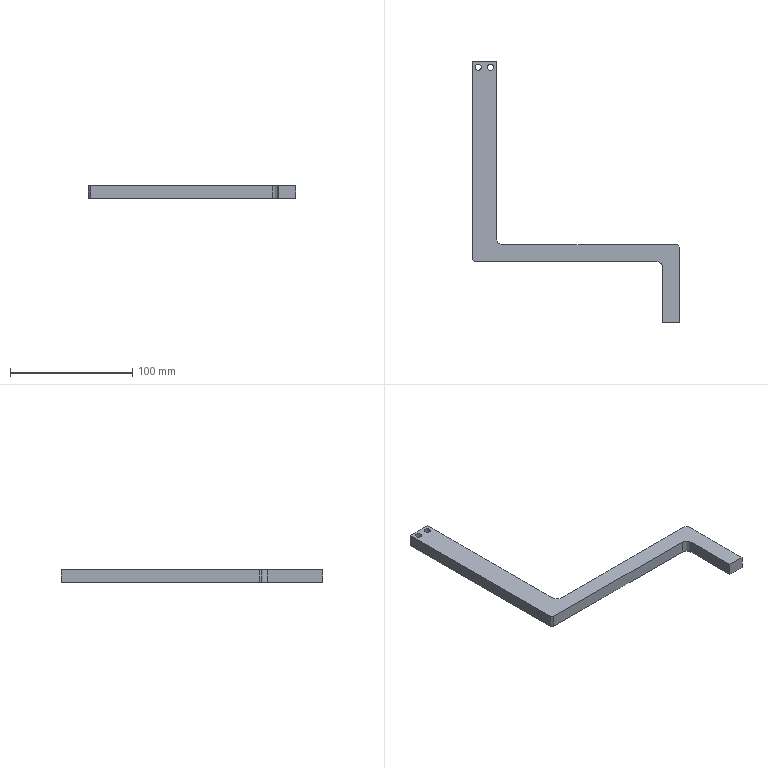Part | SolidWorks | features ICE 2, Chamfer 1, Extrusion 1, Fillet 1 | 1 solid | 18 faces | box 170 x 214 x 10 mm | volume 60475 mm3 | plane 12 | cylinder 6 | commonest cylinder face diameters 5 x4 10 x2
STEP:
#1=CARTESIAN_POINT('',(-82.5,159.,-5.));
#2=VERTEX_POINT('',#1);
#3=CARTESIAN_POINT('',(-77.5,159.,-5.));
#4=VERTEX_POINT('',#3);
#5=CARTESIAN_POINT('',(-80.,159.,-5.));
#6=DIRECTION('',(0.,0.,1.));
#7=DIRECTION('',(-1.,0.,0.));
#8=AXIS2_PLACEMENT_3D('',#5,#6,#7);
#9=CIRCLE('',#8,2.5);
#10=EDGE_CURVE('',#2,#4,#9,.T.);
#11=ORIENTED_EDGE('',*,*,#10,.F.);
#12=CARTESIAN_POINT('',(-82.5,159.,5.));
#13=VERTEX_POINT('',#12);
#14=CARTESIAN_POINT('',(-82.5,159.,-5.001));
#15=DIRECTION('',(0.,0.,1.));
#16=VECTOR('',#15,1000.);
#17=LINE('',#14,#16);
#18=EDGE_CURVE('',#2,#13,#17,.T.);
#19=ORIENTED_EDGE('',*,*,#18,.T.);
#20=CARTESIAN_POINT('',(-77.5,159.,5.));
#21=VERTEX_POINT('',#20);
#22=CARTESIAN_POINT('',(-80.,159.,5.));
#23=DIRECTION('',(0.,0.,1.));
#24=DIRECTION('',(1.,0.,0.));
#25=AXIS2_PLACEMENT_3D('',#22,#23,#24);
#26=CIRCLE('',#25,2.5);
#27=EDGE_CURVE('',#13,#21,#26,.T.);
#28=ORIENTED_EDGE('',*,*,#27,.T.);
#29=CARTESIAN_POINT('',(-77.5,159.,-5.001));
#30=DIRECTION('',(0.,0.,1.));
#31=VECTOR('',#30,1000.);
#32=LINE('',#29,#31);
#33=EDGE_CURVE('',#4,#21,#32,.T.);
#34=ORIENTED_EDGE('',*,*,#33,.F.);
#35=EDGE_LOOP('',(#11,#19,#28,#34));
#36=FACE_OUTER_BOUND('',#35,.T.);
#37=CARTESIAN_POINT('',(-80.,159.,-5.001));
#38=DIRECTION('',(0.,0.,1.));
#39=DIRECTION('',(1.,0.,0.));
#40=AXIS2_PLACEMENT_3D('',#37,#38,#39);
#41=CYLINDRICAL_SURFACE('',#40,2.5);
#42=ADVANCED_FACE('',(#36),#41,.F.);
#43=CARTESIAN_POINT('',(-72.5,159.,-5.));
#44=VERTEX_POINT('',#43);
#45=CARTESIAN_POINT('',(-67.5,159.,-5.));
#46=VERTEX_POINT('',#45);
#47=CARTESIAN_POINT('',(-70.,159.,-5.));
#48=DIRECTION('',(0.,0.,1.));
#49=DIRECTION('',(-1.,0.,0.));
#50=AXIS2_PLACEMENT_3D('',#47,#48,#49);
#51=CIRCLE('',#50,2.5);
#52=EDGE_CURVE('',#44,#46,#51,.T.);
#53=ORIENTED_EDGE('',*,*,#52,.F.);
#54=CARTESIAN_POINT('',(-72.5,159.,5.));
#55=VERTEX_POINT('',#54);
#56=CARTESIAN_POINT('',(-72.5,159.,-5.001));
#57=DIRECTION('',(0.,0.,1.));
#58=VECTOR('',#57,1000.);
#59=LINE('',#56,#58);
#60=EDGE_CURVE('',#44,#55,#59,.T.);
#61=ORIENTED_EDGE('',*,*,#60,.T.);
#62=CARTESIAN_POINT('',(-67.5,159.,5.));
#63=VERTEX_POINT('',#62);
#64=CARTESIAN_POINT('',(-70.,159.,5.));
#65=DIRECTION('',(0.,0.,1.));
#66=DIRECTION('',(1.,0.,0.));
#67=AXIS2_PLACEMENT_3D('',#64,#65,#66);
#68=CIRCLE('',#67,2.5);
#69=EDGE_CURVE('',#55,#63,#68,.T.);
#70=ORIENTED_EDGE('',*,*,#69,.T.);
#71=CARTESIAN_POINT('',(-67.5,159.,-5.001));
#72=DIRECTION('',(0.,0.,1.));
#73=VECTOR('',#72,1000.);
#74=LINE('',#71,#73);
#75=EDGE_CURVE('',#46,#63,#74,.T.);
#76=ORIENTED_EDGE('',*,*,#75,.F.);
#77=EDGE_LOOP('',(#53,#61,#70,#76));
#78=FACE_OUTER_BOUND('',#77,.T.);
#79=CARTESIAN_POINT('',(-70.,159.,-5.001));
#80=DIRECTION('',(0.,0.,1.));
#81=DIRECTION('',(1.,0.,0.));
#82=AXIS2_PLACEMENT_3D('',#79,#80,#81);
#83=CYLINDRICAL_SURFACE('',#82,2.5);
#84=ADVANCED_FACE('',(#78),#83,.F.);
#85=CARTESIAN_POINT('',(85.,-50.,-5.));
#86=VERTEX_POINT('',#85);
#87=CARTESIAN_POINT('',(85.,12.,-5.));
#88=VERTEX_POINT('',#87);
#89=CARTESIAN_POINT('',(85.,14.,-5.));
#90=DIRECTION('',(0.,1.,0.));
#91=VECTOR('',#90,1000.);
#92=LINE('',#89,#91);
#93=EDGE_CURVE('',#86,#88,#92,.T.);
#94=ORIENTED_EDGE('',*,*,#93,.T.);
#95=CARTESIAN_POINT('',(85.,12.,5.));
#96=VERTEX_POINT('',#95);
#97=CARTESIAN_POINT('',(85.,12.,5.));
#98=DIRECTION('',(0.,0.,1.));
#99=VECTOR('',#98,1000.);
#100=LINE('',#97,#99);
#101=EDGE_CURVE('',#88,#96,#100,.T.);
#102=ORIENTED_EDGE('',*,*,#101,.T.);
#103=CARTESIAN_POINT('',(85.,-50.,5.));
#104=VERTEX_POINT('',#103);
#105=CARTESIAN_POINT('',(85.,14.,5.));
#106=DIRECTION('',(0.,1.,0.));
#107=VECTOR('',#106,1000.);
#108=LINE('',#105,#107);
#109=EDGE_CURVE('',#104,#96,#108,.T.);
#110=ORIENTED_EDGE('',*,*,#109,.F.);
#111=CARTESIAN_POINT('',(85.,-50.,-56.923));
#112=DIRECTION('',(0.,0.,1.));
#113=VECTOR('',#112,1000.);
#114=LINE('',#111,#113);
#115=EDGE_CURVE('',#86,#104,#114,.T.);
#116=ORIENTED_EDGE('',*,*,#115,.F.);
#117=EDGE_LOOP('',(#94,#102,#110,#116));
#118=FACE_OUTER_BOUND('',#117,.T.);
#119=CARTESIAN_POINT('',(85.,14.,5.));
#120=DIRECTION('',(-1.,0.,0.));
#121=DIRECTION('',(0.,0.,1.));
#122=AXIS2_PLACEMENT_3D('',#119,#120,#121);
#123=PLANE('',#122);
#124=ADVANCED_FACE('',(#118),#123,.F.);
#125=CARTESIAN_POINT('',(83.,14.,5.));
#126=VERTEX_POINT('',#125);
#127=CARTESIAN_POINT('',(-60.,14.,5.));
#128=VERTEX_POINT('',#127);
#129=CARTESIAN_POINT('',(-65.,14.,5.));
#130=DIRECTION('',(-1.,0.,0.));
#131=VECTOR('',#130,1000.);
#132=LINE('',#129,#131);
#133=EDGE_CURVE('',#126,#128,#132,.T.);
#134=ORIENTED_EDGE('',*,*,#133,.F.);
#135=CARTESIAN_POINT('',(83.,14.,-5.));
#136=VERTEX_POINT('',#135);
#137=CARTESIAN_POINT('',(83.,14.,5.));
#138=DIRECTION('',(0.,0.,-1.));
#139=VECTOR('',#138,1000.);
#140=LINE('',#137,#139);
#141=EDGE_CURVE('',#126,#136,#140,.T.);
#142=ORIENTED_EDGE('',*,*,#141,.T.);
#143=CARTESIAN_POINT('',(-60.,14.,-5.));
#144=VERTEX_POINT('',#143);
#145=CARTESIAN_POINT('',(-65.,14.,-5.));
#146=DIRECTION('',(-1.,0.,0.));
#147=VECTOR('',#146,1000.);
#148=LINE('',#145,#147);
#149=EDGE_CURVE('',#136,#144,#148,.T.);
#150=ORIENTED_EDGE('',*,*,#149,.T.);
#151=CARTESIAN_POINT('',(-60.,14.,5.));
#152=DIRECTION('',(0.,0.,1.));
#153=VECTOR('',#152,1000.);
#154=LINE('',#151,#153);
#155=EDGE_CURVE('',#144,#128,#154,.T.);
#156=ORIENTED_EDGE('',*,*,#155,.T.);
#157=EDGE_LOOP('',(#134,#142,#150,#156));
#158=FACE_OUTER_BOUND('',#157,.T.);
#159=CARTESIAN_POINT('',(-65.,14.,5.));
#160=DIRECTION('',(0.,-1.,0.));
#161=DIRECTION('',(1.,0.,0.));
#162=AXIS2_PLACEMENT_3D('',#159,#160,#161);
#163=PLANE('',#162);
#164=ADVANCED_FACE('',(#158),#163,.F.);
#165=CARTESIAN_POINT('',(-65.,19.,5.));
#166=VERTEX_POINT('',#165);
#167=CARTESIAN_POINT('',(-65.,164.,5.));
#168=VERTEX_POINT('',#167);
#169=CARTESIAN_POINT('',(-65.,164.,5.));
#170=DIRECTION('',(0.,1.,0.));
#171=VECTOR('',#170,1000.);
#172=LINE('',#169,#171);
#173=EDGE_CURVE('',#166,#168,#172,.T.);
#174=ORIENTED_EDGE('',*,*,#173,.F.);
#175=CARTESIAN_POINT('',(-65.,19.,-5.));
#176=VERTEX_POINT('',#175);
#177=CARTESIAN_POINT('',(-65.,19.,-5.));
#178=DIRECTION('',(0.,0.,-1.));
#179=VECTOR('',#178,1000.);
#180=LINE('',#177,#179);
#181=EDGE_CURVE('',#166,#176,#180,.T.);
#182=ORIENTED_EDGE('',*,*,#181,.T.);
#183=CARTESIAN_POINT('',(-65.,164.,-5.));
#184=VERTEX_POINT('',#183);
#185=CARTESIAN_POINT('',(-65.,164.,-5.));
#186=DIRECTION('',(0.,1.,0.));
#187=VECTOR('',#186,1000.);
#188=LINE('',#185,#187);
#189=EDGE_CURVE('',#176,#184,#188,.T.);
#190=ORIENTED_EDGE('',*,*,#189,.T.);
#191=CARTESIAN_POINT('',(-65.,164.,5.));
#192=DIRECTION('',(0.,0.,-1.));
#193=VECTOR('',#192,1000.);
#194=LINE('',#191,#193);
#195=EDGE_CURVE('',#168,#184,#194,.T.);
#196=ORIENTED_EDGE('',*,*,#195,.F.);
#197=EDGE_LOOP('',(#174,#182,#190,#196));
#198=FACE_OUTER_BOUND('',#197,.T.);
#199=CARTESIAN_POINT('',(-65.,164.,5.));
#200=DIRECTION('',(-1.,0.,0.));
#201=DIRECTION('',(0.,-1.,0.));
#202=AXIS2_PLACEMENT_3D('',#199,#200,#201);
#203=PLANE('',#202);
#204=ADVANCED_FACE('',(#198),#203,.F.);
#205=CARTESIAN_POINT('',(-85.,164.,-5.));
#206=VERTEX_POINT('',#205);
#207=CARTESIAN_POINT('',(-85.,164.,-5.));
#208=DIRECTION('',(-1.,0.,0.));
#209=VECTOR('',#208,1000.);
#210=LINE('',#207,#209);
#211=EDGE_CURVE('',#184,#206,#210,.T.);
#212=ORIENTED_EDGE('',*,*,#211,.T.);
#213=CARTESIAN_POINT('',(-85.,164.,5.));
#214=VERTEX_POINT('',#213);
#215=CARTESIAN_POINT('',(-85.,164.,5.));
#216=DIRECTION('',(0.,0.,-1.));
#217=VECTOR('',#216,1000.);
#218=LINE('',#215,#217);
#219=EDGE_CURVE('',#214,#206,#218,.T.);
#220=ORIENTED_EDGE('',*,*,#219,.F.);
#221=CARTESIAN_POINT('',(-85.,164.,5.));
#222=DIRECTION('',(-1.,0.,0.));
#223=VECTOR('',#222,1000.);
#224=LINE('',#221,#223);
#225=EDGE_CURVE('',#168,#214,#224,.T.);
#226=ORIENTED_EDGE('',*,*,#225,.F.);
#227=ORIENTED_EDGE('',*,*,#195,.T.);
#228=EDGE_LOOP('',(#212,#220,#226,#227));
#229=FACE_OUTER_BOUND('',#228,.T.);
#230=CARTESIAN_POINT('',(-85.,164.,5.));
#231=DIRECTION('',(0.,-1.,0.));
#232=DIRECTION('',(0.,0.,-1.));
#233=AXIS2_PLACEMENT_3D('',#230,#231,#232);
#234=PLANE('',#233);
#235=ADVANCED_FACE('',(#229),#234,.F.);
#236=CARTESIAN_POINT('',(-85.,2.,-5.));
#237=VERTEX_POINT('',#236);
#238=CARTESIAN_POINT('',(-85.,0.,-5.));
#239=DIRECTION('',(0.,-1.,0.));
#240=VECTOR('',#239,1000.);
#241=LINE('',#238,#240);
#242=EDGE_CURVE('',#206,#237,#241,.T.);
#243=ORIENTED_EDGE('',*,*,#242,.T.);
#244=CARTESIAN_POINT('',(-85.,2.,5.));
#245=VERTEX_POINT('',#244);
#246=CARTESIAN_POINT('',(-85.,2.,5.));
#247=DIRECTION('',(0.,0.,1.));
#248=VECTOR('',#247,1000.);
#249=LINE('',#246,#248);
#250=EDGE_CURVE('',#237,#245,#249,.T.);
#251=ORIENTED_EDGE('',*,*,#250,.T.);
#252=CARTESIAN_POINT('',(-85.,0.,5.));
#253=DIRECTION('',(0.,-1.,0.));
#254=VECTOR('',#253,1000.);
#255=LINE('',#252,#254);
#256=EDGE_CURVE('',#214,#245,#255,.T.);
#257=ORIENTED_EDGE('',*,*,#256,.F.);
#258=ORIENTED_EDGE('',*,*,#219,.T.);
#259=EDGE_LOOP('',(#243,#251,#257,#258));
#260=FACE_OUTER_BOUND('',#259,.T.);
#261=CARTESIAN_POINT('',(-85.,0.,5.));
#262=DIRECTION('',(1.,0.,0.));
#263=DIRECTION('',(0.,0.,-1.));
#264=AXIS2_PLACEMENT_3D('',#261,#262,#263);
#265=PLANE('',#264);
#266=ADVANCED_FACE('',(#260),#265,.F.);
#267=CARTESIAN_POINT('',(-83.,0.,5.));
#268=VERTEX_POINT('',#267);
#269=CARTESIAN_POINT('',(66.,0.,5.));
#270=VERTEX_POINT('',#269);
#271=CARTESIAN_POINT('',(85.,0.,5.));
#272=DIRECTION('',(1.,0.,0.));
#273=VECTOR('',#272,1000.);
#274=LINE('',#271,#273);
#275=EDGE_CURVE('',#268,#270,#274,.T.);
#276=ORIENTED_EDGE('',*,*,#275,.F.);
#277=CARTESIAN_POINT('',(-83.,0.,-5.));
#278=VERTEX_POINT('',#277);
#279=CARTESIAN_POINT('',(-83.,0.,5.));
#280=DIRECTION('',(0.,0.,-1.));
#281=VECTOR('',#280,1000.);
#282=LINE('',#279,#281);
#283=EDGE_CURVE('',#268,#278,#282,.T.);
#284=ORIENTED_EDGE('',*,*,#283,.T.);
#285=CARTESIAN_POINT('',(66.,0.,-5.));
#286=VERTEX_POINT('',#285);
#287=CARTESIAN_POINT('',(0.,0.,-5.));
#288=DIRECTION('',(1.,0.,0.));
#289=VECTOR('',#288,1000.);
#290=LINE('',#287,#289);
#291=EDGE_CURVE('',#278,#286,#290,.T.);
#292=ORIENTED_EDGE('',*,*,#291,.T.);
#293=CARTESIAN_POINT('',(66.,0.,5.));
#294=DIRECTION('',(0.,0.,1.));
#295=VECTOR('',#294,1000.);
#296=LINE('',#293,#295);
#297=EDGE_CURVE('',#286,#270,#296,.T.);
#298=ORIENTED_EDGE('',*,*,#297,.T.);
#299=EDGE_LOOP('',(#276,#284,#292,#298));
#300=FACE_OUTER_BOUND('',#299,.T.);
#301=CARTESIAN_POINT('',(0.,0.,5.));
#302=DIRECTION('',(0.,1.,0.));
#303=DIRECTION('',(-1.,0.,0.));
#304=AXIS2_PLACEMENT_3D('',#301,#302,#303);
#305=PLANE('',#304);
#306=ADVANCED_FACE('',(#300),#305,.F.);
#307=CARTESIAN_POINT('',(-80.,159.,5.));
#308=DIRECTION('',(0.,0.,1.));
#309=DIRECTION('',(1.,0.,0.));
#310=AXIS2_PLACEMENT_3D('',#307,#308,#309);
#311=CIRCLE('',#310,2.5);
#312=EDGE_CURVE('',#21,#13,#311,.T.);
#313=ORIENTED_EDGE('',*,*,#312,.F.);
#314=ORIENTED_EDGE('',*,*,#27,.F.);
#315=EDGE_LOOP('',(#313,#314));
#316=FACE_BOUND('',#315,.T.);
#317=CARTESIAN_POINT('',(-70.,159.,5.));
#318=DIRECTION('',(0.,0.,1.));
#319=DIRECTION('',(1.,0.,0.));
#320=AXIS2_PLACEMENT_3D('',#317,#318,#319);
#321=CIRCLE('',#320,2.5);
#322=EDGE_CURVE('',#63,#55,#321,.T.);
#323=ORIENTED_EDGE('',*,*,#322,.F.);
#324=ORIENTED_EDGE('',*,*,#69,.F.);
#325=EDGE_LOOP('',(#323,#324));
#326=FACE_BOUND('',#325,.T.);
#327=ORIENTED_EDGE('',*,*,#256,.T.);
#328=CARTESIAN_POINT('',(-83.,0.,5.));
#329=DIRECTION('',(0.7071,-0.7071,0.));
#330=VECTOR('',#329,1000.);
#331=LINE('',#328,#330);
#332=EDGE_CURVE('',#245,#268,#331,.T.);
#333=ORIENTED_EDGE('',*,*,#332,.T.);
#334=ORIENTED_EDGE('',*,*,#275,.T.);
#335=CARTESIAN_POINT('',(71.,-5.,5.));
#336=VERTEX_POINT('',#335);
#337=CARTESIAN_POINT('',(66.,-5.,5.));
#338=DIRECTION('',(0.,0.,-1.));
#339=DIRECTION('',(-1.,0.,0.));
#340=AXIS2_PLACEMENT_3D('',#337,#338,#339);
#341=CIRCLE('',#340,5.);
#342=EDGE_CURVE('',#270,#336,#341,.T.);
#343=ORIENTED_EDGE('',*,*,#342,.T.);
#344=CARTESIAN_POINT('',(71.,-50.,5.));
#345=VERTEX_POINT('',#344);
#346=CARTESIAN_POINT('',(71.,0.,5.));
#347=DIRECTION('',(0.,-1.,0.));
#348=VECTOR('',#347,1000.);
#349=LINE('',#346,#348);
#350=EDGE_CURVE('',#336,#345,#349,.T.);
#351=ORIENTED_EDGE('',*,*,#350,.T.);
#352=CARTESIAN_POINT('',(85.,-50.,5.));
#353=DIRECTION('',(1.,0.,0.));
#354=VECTOR('',#353,1000.);
#355=LINE('',#352,#354);
#356=EDGE_CURVE('',#345,#104,#355,.T.);
#357=ORIENTED_EDGE('',*,*,#356,.T.);
#358=ORIENTED_EDGE('',*,*,#109,.T.);
#359=CARTESIAN_POINT('',(83.,14.,5.));
#360=DIRECTION('',(-0.7071,0.7071,0.));
#361=VECTOR('',#360,1000.);
#362=LINE('',#359,#361);
#363=EDGE_CURVE('',#96,#126,#362,.T.);
#364=ORIENTED_EDGE('',*,*,#363,.T.);
#365=ORIENTED_EDGE('',*,*,#133,.T.);
#366=CARTESIAN_POINT('',(-60.,19.,5.));
#367=DIRECTION('',(0.,0.,-1.));
#368=DIRECTION('',(-1.,0.,0.));
#369=AXIS2_PLACEMENT_3D('',#366,#367,#368);
#370=CIRCLE('',#369,5.);
#371=EDGE_CURVE('',#128,#166,#370,.T.);
#372=ORIENTED_EDGE('',*,*,#371,.T.);
#373=ORIENTED_EDGE('',*,*,#173,.T.);
#374=ORIENTED_EDGE('',*,*,#225,.T.);
#375=EDGE_LOOP('',(#327,#333,#334,#343,#351,#357,#358,#364,#365,#372,#373,#374));
#376=FACE_OUTER_BOUND('',#375,.T.);
#377=CARTESIAN_POINT('',(0.,0.,5.));
#378=DIRECTION('',(0.,0.,-1.));
#379=DIRECTION('',(-1.,0.,0.));
#380=AXIS2_PLACEMENT_3D('',#377,#378,#379);
#381=PLANE('',#380);
#382=ADVANCED_FACE('',(#316,#326,#376),#381,.F.);
#383=CARTESIAN_POINT('',(-80.,159.,-5.));
#384=DIRECTION('',(0.,0.,1.));
#385=DIRECTION('',(-1.,0.,0.));
#386=AXIS2_PLACEMENT_3D('',#383,#384,#385);
#387=CIRCLE('',#386,2.5);
#388=EDGE_CURVE('',#4,#2,#387,.T.);
#389=ORIENTED_EDGE('',*,*,#388,.T.);
#390=ORIENTED_EDGE('',*,*,#10,.T.);
#391=EDGE_LOOP('',(#389,#390));
#392=FACE_BOUND('',#391,.T.);
#393=CARTESIAN_POINT('',(-70.,159.,-5.));
#394=DIRECTION('',(0.,0.,1.));
#395=DIRECTION('',(-1.,0.,0.));
#396=AXIS2_PLACEMENT_3D('',#393,#394,#395);
#397=CIRCLE('',#396,2.5);
#398=EDGE_CURVE('',#46,#44,#397,.T.);
#399=ORIENTED_EDGE('',*,*,#398,.T.);
#400=ORIENTED_EDGE('',*,*,#52,.T.);
#401=EDGE_LOOP('',(#399,#400));
#402=FACE_BOUND('',#401,.T.);
#403=ORIENTED_EDGE('',*,*,#291,.F.);
#404=CARTESIAN_POINT('',(-41.5,-41.5,-5.));
#405=DIRECTION('',(-0.7071,0.7071,0.));
#406=VECTOR('',#405,1000.);
#407=LINE('',#404,#406);
#408=EDGE_CURVE('',#278,#237,#407,.T.);
#409=ORIENTED_EDGE('',*,*,#408,.T.);
#410=ORIENTED_EDGE('',*,*,#242,.F.);
#411=ORIENTED_EDGE('',*,*,#211,.F.);
#412=ORIENTED_EDGE('',*,*,#189,.F.);
#413=CARTESIAN_POINT('',(-60.,19.,-5.));
#414=DIRECTION('',(0.,0.,1.));
#415=DIRECTION('',(-1.,0.,0.));
#416=AXIS2_PLACEMENT_3D('',#413,#414,#415);
#417=CIRCLE('',#416,5.);
#418=EDGE_CURVE('',#176,#144,#417,.T.);
#419=ORIENTED_EDGE('',*,*,#418,.T.);
#420=ORIENTED_EDGE('',*,*,#149,.F.);
#421=CARTESIAN_POINT('',(48.5,48.5,-5.));
#422=DIRECTION('',(0.7071,-0.7071,0.));
#423=VECTOR('',#422,1000.);
#424=LINE('',#421,#423);
#425=EDGE_CURVE('',#136,#88,#424,.T.);
#426=ORIENTED_EDGE('',*,*,#425,.T.);
#427=ORIENTED_EDGE('',*,*,#93,.F.);
#428=CARTESIAN_POINT('',(71.,-50.,-5.));
#429=VERTEX_POINT('',#428);
#430=CARTESIAN_POINT('',(85.,-50.,-5.));
#431=DIRECTION('',(1.,0.,0.));
#432=VECTOR('',#431,1000.);
#433=LINE('',#430,#432);
#434=EDGE_CURVE('',#429,#86,#433,.T.);
#435=ORIENTED_EDGE('',*,*,#434,.F.);
#436=CARTESIAN_POINT('',(71.,-5.,-5.));
#437=VERTEX_POINT('',#436);
#438=CARTESIAN_POINT('',(71.,0.,-5.));
#439=DIRECTION('',(0.,-1.,0.));
#440=VECTOR('',#439,1000.);
#441=LINE('',#438,#440);
#442=EDGE_CURVE('',#437,#429,#441,.T.);
#443=ORIENTED_EDGE('',*,*,#442,.F.);
#444=CARTESIAN_POINT('',(66.,-5.,-5.));
#445=DIRECTION('',(0.,0.,1.));
#446=DIRECTION('',(-1.,0.,0.));
#447=AXIS2_PLACEMENT_3D('',#444,#445,#446);
#448=CIRCLE('',#447,5.);
#449=EDGE_CURVE('',#437,#286,#448,.T.);
#450=ORIENTED_EDGE('',*,*,#449,.T.);
#451=EDGE_LOOP('',(#403,#409,#410,#411,#412,#419,#420,#426,#427,#435,#443,#450));
#452=FACE_OUTER_BOUND('',#451,.T.);
#453=CARTESIAN_POINT('',(0.,0.,-5.));
#454=DIRECTION('',(0.,0.,-1.));
#455=DIRECTION('',(-1.,0.,0.));
#456=AXIS2_PLACEMENT_3D('',#453,#454,#455);
#457=PLANE('',#456);
#458=ADVANCED_FACE('',(#392,#402,#452),#457,.T.);
#459=ORIENTED_EDGE('',*,*,#60,.F.);
#460=ORIENTED_EDGE('',*,*,#398,.F.);
#461=ORIENTED_EDGE('',*,*,#75,.T.);
#462=ORIENTED_EDGE('',*,*,#322,.T.);
#463=EDGE_LOOP('',(#459,#460,#461,#462));
#464=FACE_OUTER_BOUND('',#463,.T.);
#465=CARTESIAN_POINT('',(-70.,159.,-5.001));
#466=DIRECTION('',(0.,0.,1.));
#467=DIRECTION('',(1.,0.,0.));
#468=AXIS2_PLACEMENT_3D('',#465,#466,#467);
#469=CYLINDRICAL_SURFACE('',#468,2.5);
#470=ADVANCED_FACE('',(#464),#469,.F.);
#471=ORIENTED_EDGE('',*,*,#18,.F.);
#472=ORIENTED_EDGE('',*,*,#388,.F.);
#473=ORIENTED_EDGE('',*,*,#33,.T.);
#474=ORIENTED_EDGE('',*,*,#312,.T.);
#475=EDGE_LOOP('',(#471,#472,#473,#474));
#476=FACE_OUTER_BOUND('',#475,.T.);
#477=CARTESIAN_POINT('',(-80.,159.,-5.001));
#478=DIRECTION('',(0.,0.,1.));
#479=DIRECTION('',(1.,0.,0.));
#480=AXIS2_PLACEMENT_3D('',#477,#478,#479);
#481=CYLINDRICAL_SURFACE('',#480,2.5);
#482=ADVANCED_FACE('',(#476),#481,.F.);
#483=ORIENTED_EDGE('',*,*,#350,.F.);
#484=CARTESIAN_POINT('',(71.,-5.,-56.923));
#485=DIRECTION('',(0.,0.,-1.));
#486=VECTOR('',#485,1000.);
#487=LINE('',#484,#486);
#488=EDGE_CURVE('',#336,#437,#487,.T.);
#489=ORIENTED_EDGE('',*,*,#488,.T.);
#490=ORIENTED_EDGE('',*,*,#442,.T.);
#491=CARTESIAN_POINT('',(71.,-50.,-56.923));
#492=DIRECTION('',(0.,0.,1.));
#493=VECTOR('',#492,1000.);
#494=LINE('',#491,#493);
#495=EDGE_CURVE('',#429,#345,#494,.T.);
#496=ORIENTED_EDGE('',*,*,#495,.T.);
#497=EDGE_LOOP('',(#483,#489,#490,#496));
#498=FACE_OUTER_BOUND('',#497,.T.);
#499=CARTESIAN_POINT('',(71.,0.,-56.923));
#500=DIRECTION('',(-1.,0.,0.));
#501=DIRECTION('',(0.,0.,1.));
#502=AXIS2_PLACEMENT_3D('',#499,#500,#501);
#503=PLANE('',#502);
#504=ADVANCED_FACE('',(#498),#503,.T.);
#505=ORIENTED_EDGE('',*,*,#495,.F.);
#506=ORIENTED_EDGE('',*,*,#434,.T.);
#507=ORIENTED_EDGE('',*,*,#115,.T.);
#508=ORIENTED_EDGE('',*,*,#356,.F.);
#509=EDGE_LOOP('',(#505,#506,#507,#508));
#510=FACE_OUTER_BOUND('',#509,.T.);
#511=CARTESIAN_POINT('',(85.,-50.,-56.923));
#512=DIRECTION('',(0.,-1.,0.));
#513=DIRECTION('',(0.,0.,-1.));
#514=AXIS2_PLACEMENT_3D('',#511,#512,#513);
#515=PLANE('',#514);
#516=ADVANCED_FACE('',(#510),#515,.T.);
#517=ORIENTED_EDGE('',*,*,#371,.F.);
#518=ORIENTED_EDGE('',*,*,#155,.F.);
#519=ORIENTED_EDGE('',*,*,#418,.F.);
#520=ORIENTED_EDGE('',*,*,#181,.F.);
#521=EDGE_LOOP('',(#517,#518,#519,#520));
#522=FACE_OUTER_BOUND('',#521,.T.);
#523=CARTESIAN_POINT('',(-60.,19.,5.));
#524=DIRECTION('',(0.,0.,1.));
#525=DIRECTION('',(1.,0.,0.));
#526=AXIS2_PLACEMENT_3D('',#523,#524,#525);
#527=CYLINDRICAL_SURFACE('',#526,5.);
#528=ADVANCED_FACE('',(#522),#527,.F.);
#529=ORIENTED_EDGE('',*,*,#449,.F.);
#530=ORIENTED_EDGE('',*,*,#488,.F.);
#531=ORIENTED_EDGE('',*,*,#342,.F.);
#532=ORIENTED_EDGE('',*,*,#297,.F.);
#533=EDGE_LOOP('',(#529,#530,#531,#532));
#534=FACE_OUTER_BOUND('',#533,.T.);
#535=CARTESIAN_POINT('',(66.,-5.,5.));
#536=DIRECTION('',(0.,0.,1.));
#537=DIRECTION('',(1.,0.,0.));
#538=AXIS2_PLACEMENT_3D('',#535,#536,#537);
#539=CYLINDRICAL_SURFACE('',#538,5.);
#540=ADVANCED_FACE('',(#534),#539,.F.);
#541=ORIENTED_EDGE('',*,*,#332,.F.);
#542=ORIENTED_EDGE('',*,*,#250,.F.);
#543=ORIENTED_EDGE('',*,*,#408,.F.);
#544=ORIENTED_EDGE('',*,*,#283,.F.);
#545=EDGE_LOOP('',(#541,#542,#543,#544));
#546=FACE_OUTER_BOUND('',#545,.T.);
#547=CARTESIAN_POINT('',(-83.,0.,5.));
#548=DIRECTION('',(0.7071,0.7071,0.));
#549=DIRECTION('',(0.,0.,-1.));
#550=AXIS2_PLACEMENT_3D('',#547,#548,#549);
#551=PLANE('',#550);
#552=ADVANCED_FACE('',(#546),#551,.F.);
#553=ORIENTED_EDGE('',*,*,#363,.F.);
#554=ORIENTED_EDGE('',*,*,#101,.F.);
#555=ORIENTED_EDGE('',*,*,#425,.F.);
#556=ORIENTED_EDGE('',*,*,#141,.F.);
#557=EDGE_LOOP('',(#553,#554,#555,#556));
#558=FACE_OUTER_BOUND('',#557,.T.);
#559=CARTESIAN_POINT('',(83.,14.,5.));
#560=DIRECTION('',(-0.7071,-0.7071,0.));
#561=DIRECTION('',(0.,0.,-1.));
#562=AXIS2_PLACEMENT_3D('',#559,#560,#561);
#563=PLANE('',#562);
#564=ADVANCED_FACE('',(#558),#563,.F.);
#565=CLOSED_SHELL('',(#42,#84,#124,#164,#204,#235,#266,#306,#382,#458,#470,#482,#504,#516,#528,#540,#552,#564));
#566=MANIFOLD_SOLID_BREP('',#565);
#567=CARTESIAN_POINT('',(0.,0.,0.));
#568=DIRECTION('',(0.,0.,1.));
#569=DIRECTION('',(1.,0.,0.));
#570=AXIS2_PLACEMENT_3D('',#567,#568,#569);
#571=(LENGTH_UNIT()NAMED_UNIT(*)SI_UNIT(.MILLI.,.METRE.));
#572=UNCERTAINTY_MEASURE_WITH_UNIT(LENGTH_MEASURE(0.00001),#571,'','');
#573=(NAMED_UNIT(*)PLANE_ANGLE_UNIT()SI_UNIT($,.RADIAN.));
#574=(NAMED_UNIT(*)SI_UNIT($,.STERADIAN.)SOLID_ANGLE_UNIT());
#575=(GEOMETRIC_REPRESENTATION_CONTEXT(3)GLOBAL_UNCERTAINTY_ASSIGNED_CONTEXT((#572))GLOBAL_UNIT_ASSIGNED_CONTEXT((#571,#573,#574))REPRESENTATION_CONTEXT('',''));
#576=ADVANCED_BREP_SHAPE_REPRESENTATION('',(#566,#570),#575);